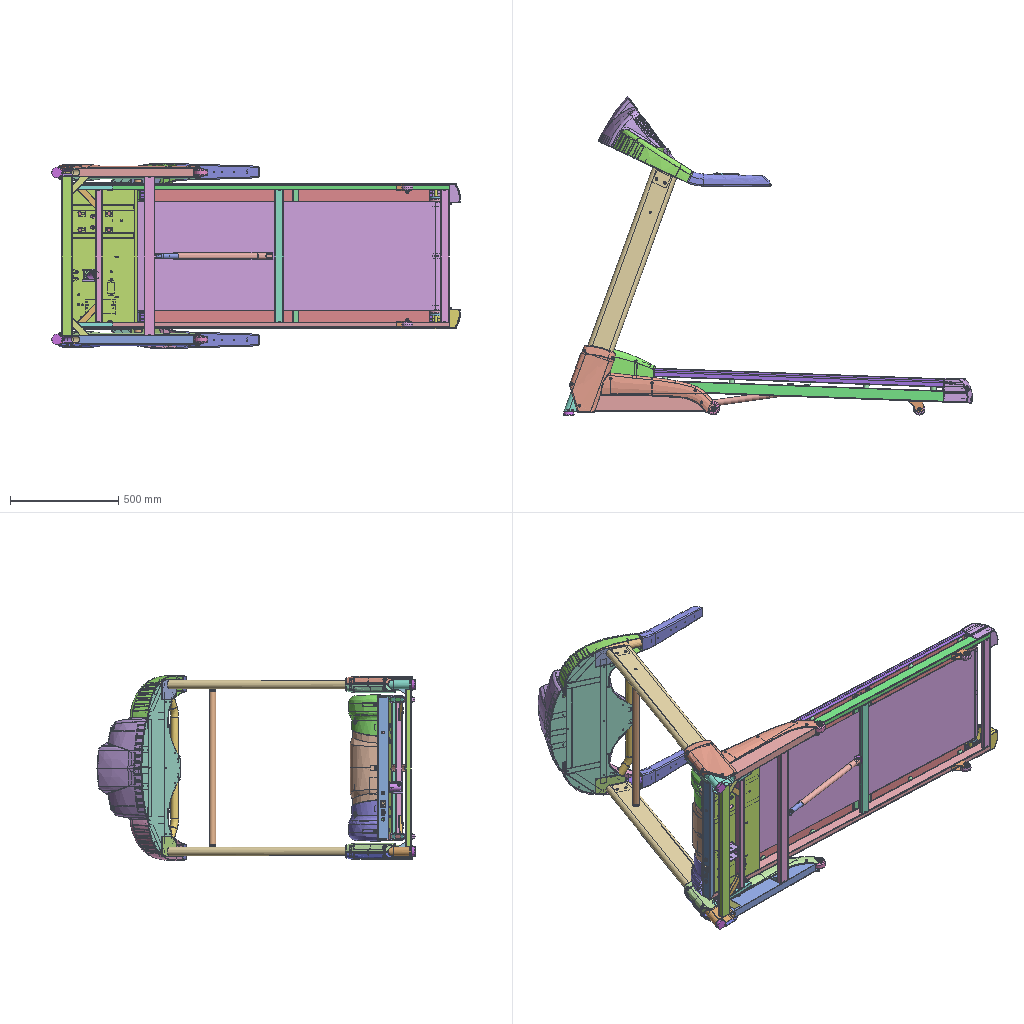Assembly | STEP file | 128 different items | 245 placed | box 1886 x 1467 x 856 mm
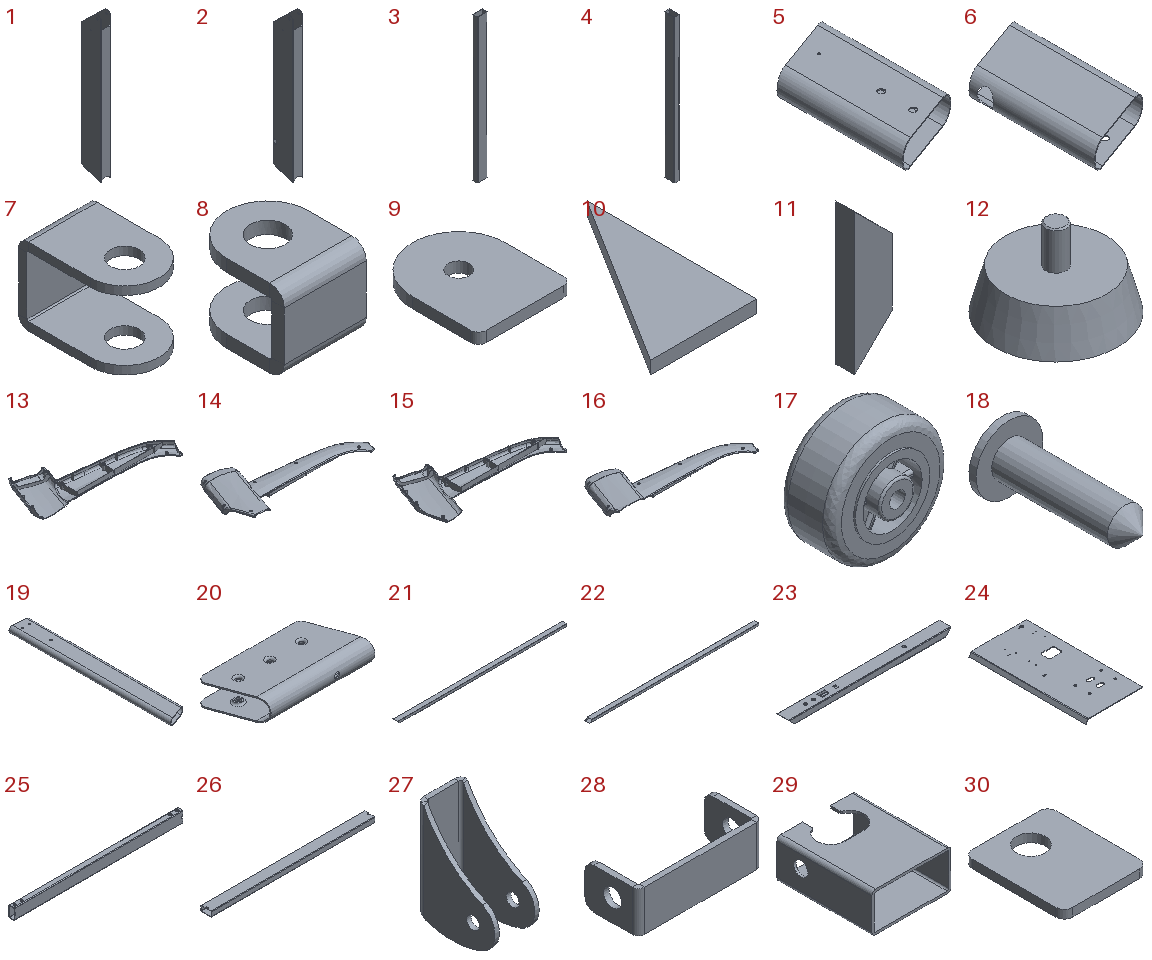Parts list (item | name | quantity | parent item | size | volume):
1 | Q7C0101L | x1 | in Q7C0100 | 40 x 80 x 584.662 mm | 247480 mm3
2 | Q7C0101R | x1 | in Q7C0100 | 40 x 80 x 584.662 mm | 247142 mm3
3 | PN_0025_default | x1 | in Q7C0100 | 50 x 25 x 730 mm | 154272 mm3
4 | PN_0006_default | x1 | in Q7C0100 | 25 x 50 x 730 mm | 154272 mm3
5 | Q7C0104L | x1 | in Q7C0100 | 120 x 240.676 x 40 mm | 82650 mm3
6 | Q7C0104R | x1 | in Q7C0100 | 120 x 240.549 x 40 mm | 81709 mm3
7 | Q7C0106 | x4 | in Q7C0100, Q7C0500 | 25 x 38.5 x 28 mm | 6374 mm3
8 | PN_0005_default | x1 | in Q7C0100 | 20 x 24 x 19 mm | 2959 mm3
9 | PN_0009_default | x2 | in Q7C0100 | 35 x 42.5 x 4 mm | 5208 mm3
10 | Q7C0109 | x4 | in Q7C0100 | 25 x 40 x 3 mm | 1500 mm3
11 | Q7C0110 | x2 | in Q7C0100 | 30 x 15 x 113 mm | 10458 mm3
12 | Q7C0102W | x2 | in Q7C0100Z | 48.593 x 48.593 x 32 mm | 27204 mm3
13 | PR12S0312~665.310.45LR | x1 | in Q7C0100Z | 660.94 x 308.881 x 43 mm | 303745 mm3
14 | PR12S0313~665.310.45LL | x1 | in Q7C0100Z | 660.94 x 308.908 x 43 mm | 328028 mm3
15 | PR12S0312~665.310.45RR | x1 | in Q7C0100Z | 660.94 x 308.908 x 43 mm | 328301 mm3
16 | PR12S0312~665.310.45RL | x1 | in Q7C0100Z | 660.94 x 308.881 x 43 mm | 302873 mm3
17 | 04FS0060~8.2.62.T35 | x2 | in Q7C0100Z | 62 x 35 x 62 mm | 74583 mm3
18 | ZG0415 | x1 | in Q7C0100Z | 7.5 x 16.961 x 7.5 mm | 227.201 mm3
19 | Q7C0201 | x2 | in Q7C0200 | 120 x 1000 x 40 mm | 489501 mm3
20 | PN_0014_default | x2 | in Q7C0200 | 192.331 x 89 x 35 mm | 64591 mm3
21 | Q7C0501L | x1 | in Q7C0500 | 1765 x 50 x 25 mm | 371060 mm3
22 | Q7C0501R | x1 | in Q7C0500 | 1765 x 50 x 25 mm | 371163 mm3
23 | Q7C0502 | x1 | in Q7C0500 | 658 x 50 x 25 mm | 125904 mm3
24 | PN_0024_default | x1 | in Q7C0500 | 299.634 x 609 x 21.187 mm | 548707 mm3
25 | Q7C0504 | x1 | in Q7C0500 | 610 x 20 x 40 mm | 101740 mm3
26 | Q7C0505 | x1 | in Q7C0500 | 610 x 40 x 20 mm | 101443 mm3
27 | Q7C0506 | x2 | in Q7C0500 | 30 x 53 x 70.522 mm | 17329 mm3
28 | Q7C0507 | x2 | in Q7C0500 | 70 x 30 x 23 mm | 7902 mm3
29 | Q7C0508 | x1 | in Q7C0500 | 50 x 60 x 25 mm | 11629 mm3
30 | Q7C0509 | x1 | in Q7C0500 | 50 x 60 x 5 mm | 13731 mm3
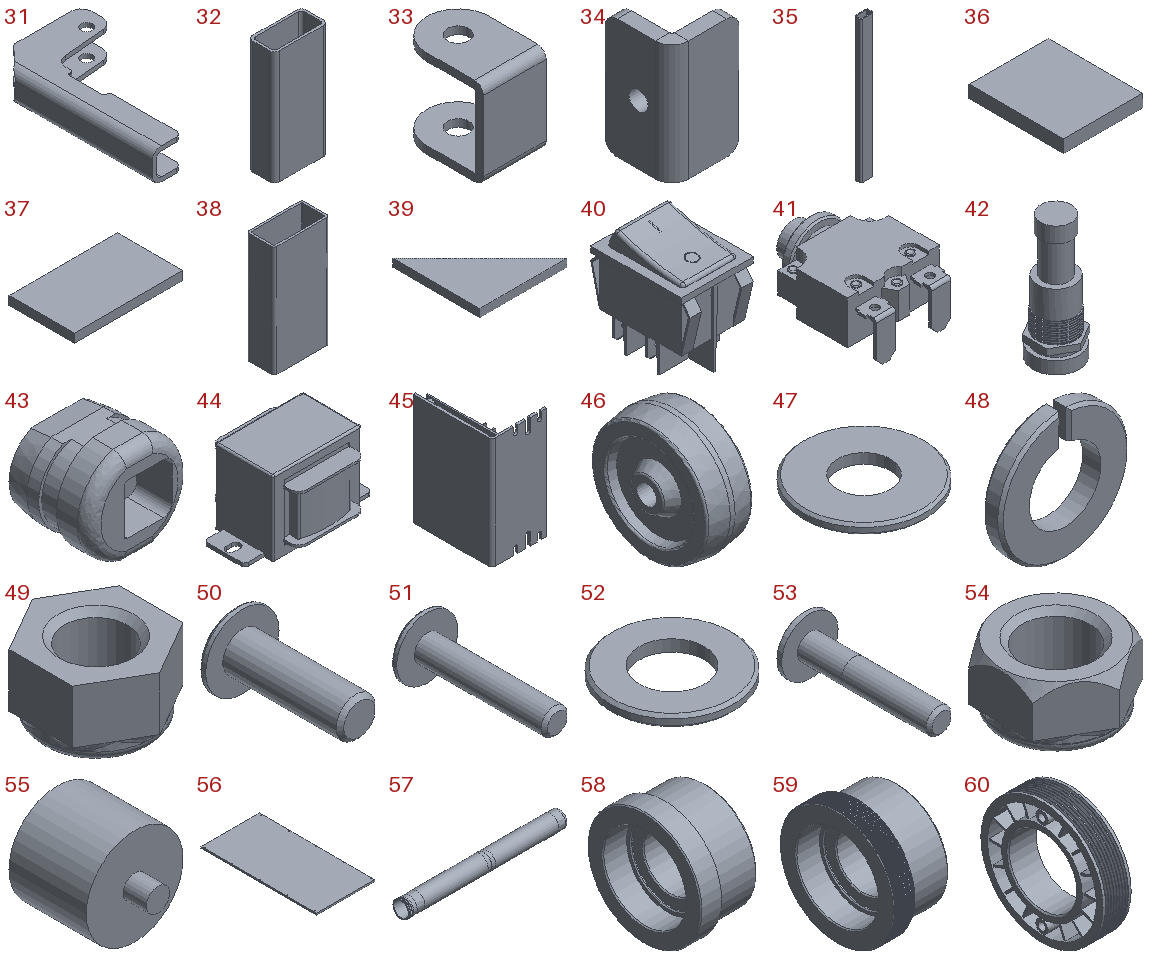31 | Q7C0510 | x1 | in Q7C0500 | 84 x 150 x 29 mm | 50454 mm3
32 | Q7C0511 | x2 | in Q7C0500 | 26 x 13 x 55 mm | 4616 mm3
33 | Q7C0512 | x1 | in Q7C0500 | 25 x 35 x 35 mm | 6553 mm3
34 | Q7C0513 | x7 | in Q7C0500 | 14 x 14 x 25 mm | 1757 mm3
35 | Q7C0515 | x2 | in Q7C0500 | 26 x 13 x 285 mm | 23919 mm3
36 | Q7C0516 | x1 | in Q7C0500 | 25 x 30 x 4 mm | 3000 mm3
37 | Q7C0518 | x2 | in Q7C0500 | 50 x 30 x 4 mm | 6000 mm3
38 | Q7C0519 | x1 | in Q7C0500 | 40 x 20 x 80 mm | 13422 mm3
39 | Q7C0517 | x2 | in Q7C0500 | 45 x 45 x 4 mm | 4050 mm3
40 | EP002 | x1 | in Q7C0500Z | 25 x 34.5 x 34.784 mm | 14567 mm3
41 | EC002 | x1 | in Q7C0500Z | 29.3 x 39.3 x 19.65 mm | 10331 mm3
42 | PN_0007_default | x1 | in Q7C0500Z | 15 x 16.018 x 40 mm | 4012 mm3
43 | PN_0016_default | x1 | in Q7C0500Z | 17 x 14 x 16 mm | 1519 mm3
44 | PN_0019-default | x1 | in Q7C0500Z | 72 x 50 x 42 mm | 79868 mm3
45 | ZY03WYF | x1 | in Q7C0500Z | 68 x 97.5 x 138 mm | 146420 mm3
46 | PN_0013_config | x2 | in Q7C0500Z | 22 x 52.843 x 52.843 mm | 34026 mm3
47 | PN_0027_config | x7 | in Q7C0500Z | 9.8 x 9.8 x 0.8 mm | 48.045 mm3
48 | W204009 | x7 | in Q7C0500Z | 9.2 x 1.3 x 9.193 mm | 57.255 mm3
49 | PN_0001_config | x8 | in Q7C0500Z | 7 x 8.083 x 4.7 mm | 129.872 mm3
50 | SD10412 | x9 | in Q7C0500Z | 9.4 x 17.503 x 9.4 mm | 388.67 mm3
51 | SD10420 | x2 | in Q7C0500Z | 9.4 x 22.503 x 9.4 mm | 345.867 mm3
52 | PN_0008_config | x5 | in Q7C0500Z | 17 x 17 x 1.6 mm | 252.969 mm3
53 | PN_0004_config | x3 | in Q7C0500Z, Q7C | 18 x 46.451 x 18 mm | 2805 mm3
54 | PN_0010_config | x2 | in Q7C0500Z | 13.017 x 15.011 x 7.5 mm | 666.866 mm3
55 | DECH01 | x8 | in Q7C0500Z | 25 x 26 x 25 mm | 9704 mm3
56 | DECAK NQ7A | x1 | in Q7C0500Z | 658 x 1310 x 18 mm | 15510409 mm3
57 | PN_0023_default | x1 | in Q7C0700ZA | 543 x 56 x 56 mm | 266273 mm3
58 | PN_0020_default | x1 | in Q7C0700ZA | 30 x 55.001 x 55.001 mm | 38129 mm3
59 | PN_0015_default | x1 | in Q7C0700ZA | 30 x 55.999 x 56 mm | 38879 mm3
60 | PN_0017_default | x1 | in Q7C0700ZA | 23 x 100 x 100 mm | 79245 mm3
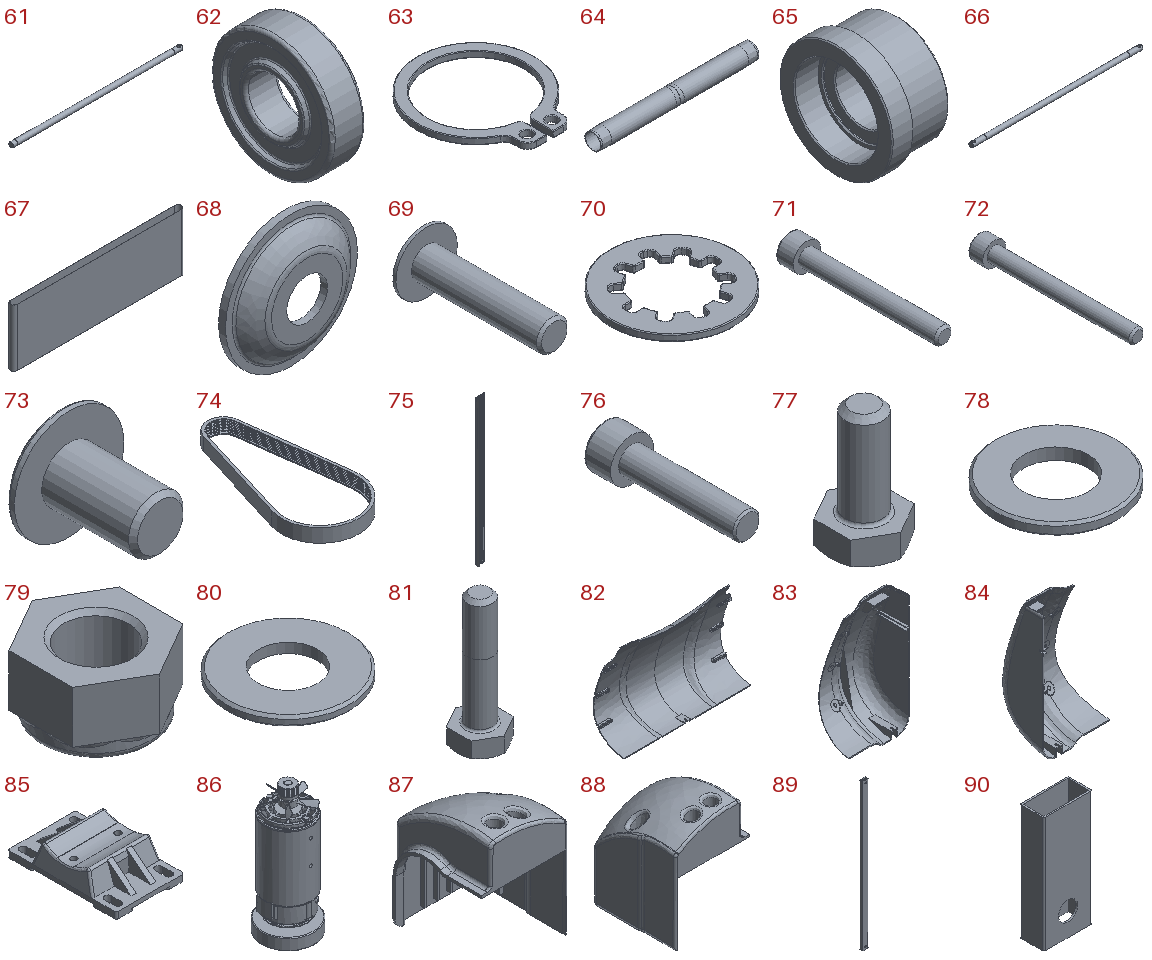61 | Q7C0702 | x1 | in Q7C0700Z | 610 x 17 x 17 mm | 138904 mm3
62 | PL6203ZZA_default | x4 | in Q7C0700Z, Q7C0800Z | 11 x 40 x 40 mm | 9892 mm3
63 | PN_0018_config | x4 | in Q7C0700Z, Q7C0800Z | 19 x 21.5 x 1 mm | 101.865 mm3
64 | PN_0012_default | x1 | in Q7C0800ZA | 530 x 56 x 56 mm | 259272 mm3
65 | PN_0003_default | x2 | in Q7C0800ZA | 30 x 54.43 x 54.43 mm | 37639 mm3
66 | Q7C0803 | x1 | in Q7C0800Z | 655 x 17 x 17 mm | 147236 mm3
67 | RUBE Q7C | x1 | in Q7C0500Z | 1492 x 59.6 x 500 mm | 2741026 mm3
68 | PN_0022_default | x6 | in Q7C0500Z | 21 x 3.607 x 21 mm | 386.807 mm3
69 | SD10625 | x8 | in Q7C0500Z | 12 x 27.352 x 12 mm | 852.352 mm3
70 | PN_0026_config | x3 | in Q7C0500Z | 15 x 15 x 0.8 mm | 82.689 mm3
71 | SA10865 | x1 | in Q7C0500Z | 13 x 73 x 13 mm | 4160 mm3
72 | SA10880 | x2 | in Q7C0500Z | 13 x 88 x 13 mm | 4914 mm3
73 | SD10610 | x5 | in Q7C0500Z | 12 x 12.964 x 12 mm | 479.053 mm3
74 | DE200JNQ7A | x1 | in Q7C0500Z | 103 x 213.3 x 18 mm | 21815 mm3
75 | SIDE-D default | x2 | in Q7C0500Z | 82 x 38 x 1350 mm | 698294 mm3
76 | SA10835 | x1 | in Q7C0500Z | 13 x 43 x 13 mm | 2660 mm3
77 | SI1025_M10 | x4 | in Q7C0500Z | 17 x 19.6 x 32 mm | 3678 mm3
78 | PN_0028_config | x5 | in Q7C0500Z | 21 x 21 x 2 mm | 492.233 mm3
79 | N210095 | x5 | in Q7C0500Z | 17 x 19.63 x 10.5 mm | 1722 mm3
80 | PN_0021_config | x1 | in Q7C0500Z | 25 x 25 x 2 mm | 736.18 mm3
81 | SI11045_M10 | x1 | in Q7C0500Z | 17 x 19.6 x 52 mm | 5249 mm3
82 | MOTOR COVER Z | x1 | in Q7C0500Z | 500 x 131.956 x 336.482 mm | 623732 mm3
83 | MOTOR COVER R | x1 | in Q7C0500Z | 191.608 x 140.54 x 371.606 mm | 329037 mm3
84 | MOTOR COVER L | x1 | in Q7C0500Z | 191.608 x 140.54 x 371.606 mm | 339460 mm3
85 | MDZ Q7A | x1 | in Q7C0600Z | 100 x 160 x 38.7 mm | 142621 mm3
86 | MOTOR Q7A | x1 | in Q7C0600Z | 142 x 142 x 347 mm | 1832785 mm3
87 | EDN CAP NQ7A | x1 | in Q7C0500Z | 100.427 x 109.896 x 135.338 mm | 139649 mm3
88 | EDN CAP NQ7AL | x1 | in Q7C0500Z | 100.427 x 109.896 x 135.338 mm | 140123 mm3
89 | Q7C0901 | x2 | in Q7C0500Z | 26 x 13 x 648 mm | 67252 mm3
90 | Q7C1201 | x2 | in Q7C1200 | 30 x 15 x 72 mm | 5997 mm3
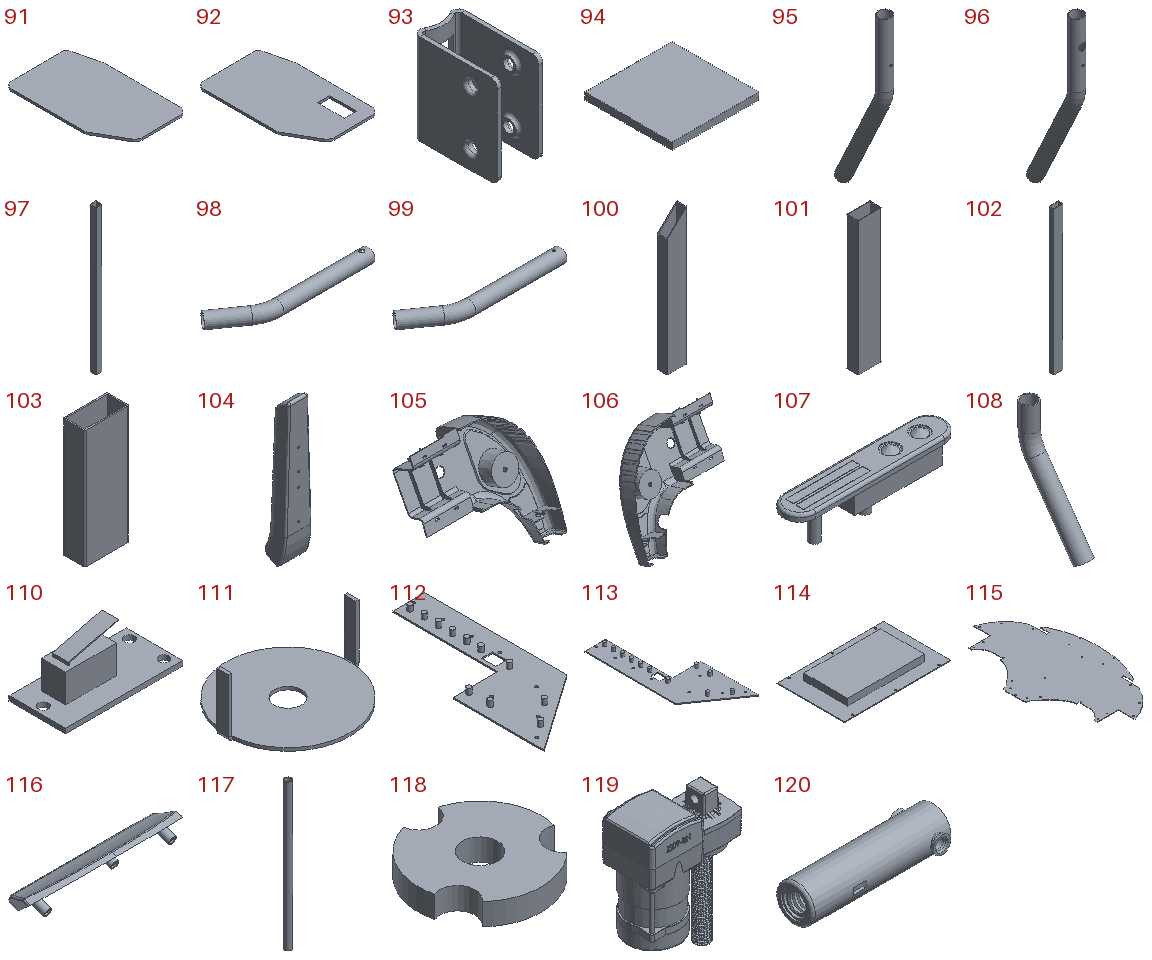91 | Q7C1202L | x1 | in Q7C1200 | 90 x 149 x 3 mm | 37856 mm3
92 | Q7C1202R | x1 | in Q7C1200 | 90 x 149 x 3 mm | 36176 mm3
93 | PN_0011_default | x2 | in Q7C1200 | 35 x 65 x 70 mm | 31433 mm3
94 | Q7C1204 | x2 | in Q7C1200 | 25 x 25 x 2 mm | 1250 mm3
95 | Q7C1205L | x1 | in Q7C1200 | 38.1 x 161.362 x 488.383 mm | 85140 mm3
96 | Q7C1205R | x1 | in Q7C1200 | 38.1 x 161.362 x 488.383 mm | 84651 mm3
97 | Q7C1206 | x1 | in Q7C1200 | 30 x 30 x 700 mm | 154296 mm3
98 | Q7C1207L | x1 | in Q7C1200 | 330.538 x 89.278 x 31.8 mm | 48236 mm3
99 | Q7C1207R | x1 | in Q7C1200 | 330.538 x 89.278 x 31.8 mm | 48237 mm3
100 | Q7C1208 | x2 | in Q7C1200 | 30 x 15 x 209.35 mm | 16574 mm3
101 | Q7C1209 | x2 | in Q7C1200 | 30 x 15 x 169 mm | 14389 mm3
102 | Q7C1210 | x1 | in Q7C1200 | 30 x 15 x 450 mm | 38263 mm3
103 | Q7C1211 | x1 | in Q7C1200 | 30 x 15 x 80 mm | 6811 mm3
104 | Handlebar Cover L | x2 | in Q7C1200ZB | 78.327 x 65.639 x 387.41 mm | 737396 mm3
105 | Consen Cover L | x1 | in Q7C1200ZB | 398.708 x 218.09 x 381.338 mm | 579816 mm3
106 | Consen Cover R | x1 | in Q7C1200ZB | 398.708 x 218.09 x 381.338 mm | 568981 mm3
107 | Q7C1216W | x2 | in Q7C1200ZB | 119.5 x 24 x 32.509 mm | 28513 mm3
108 | Q7C1217W | x2 | in Q7C1200ZB | 35.8 x 156.01 x 266.792 mm | 62409 mm3
109 | Consen Cover | x1 | in Q7C1200ZA | - | -
110 | Q7C1213W | x1 | in Q7C1200ZA | 29 x 14 x 12 mm | 1005 mm3
111 | Q7C1215W | x1 | in Q7C1200ZA | 33.859 x 32 x 15.058 mm | 684.385 mm3
112 | PCB-R | x1 | in Q7C1200ZA | 108 x 276 x 10 mm | 34872 mm3
113 | PCB-L | x1 | in Q7C1200ZA | 108 x 276 x 10 mm | 34872 mm3
114 | Q7C1214W | x1 | in Q7C1200ZA | 223 x 140 x 15.5 mm | 251677 mm3
115 | Rear Consen Cover | x1 | in Q7C1200Z | 420.328 x 794.391 x 2 mm | 399134 mm3
116 | 50FAS0309~100.33.15 | x1 | in Q7C1200Z | - | -
117 | Q7C1301 | x1 | in Q7C1300 | 31.8 x 31.8 x 726 mm | 103662 mm3
118 | PN_0002_default | x2 | in Q7C1300 | 28 x 27.429 x 5 mm | 2473 mm3
119 | JS-09 Q7A | x1 | in Q7C | 127.975 x 72.828 x 177.5 mm | 665707 mm3
120 | JS09-BNB Q7A | x1 | in Q7C | 130.5 x 41.999 x 35 mm | 51748 mm3
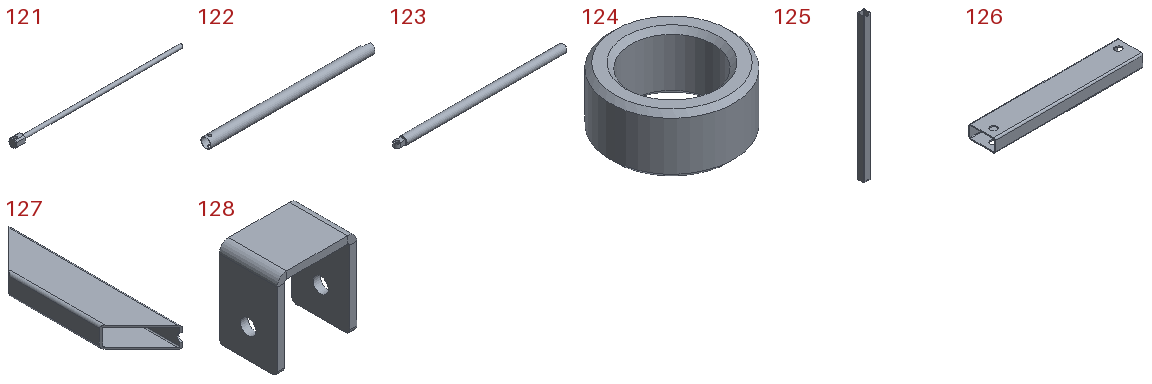121 | GAS SHOCK Q7AS | x1 | in Q7C | 478.5 x 20 x 20 mm | 44511 mm3
122 | GAS SHOCK Q7AW | x1 | in Q7C | 460 x 28 x 28 mm | 56023 mm3
123 | GAS SHOCK Q7AX | x1 | in Q7C | 474 x 22 x 22 mm | 124828 mm3
124 | Q7C0902 | x1 | in Q7C | 12.7 x 12.7 x 6 mm | 402.941 mm3
125 | PN_0030_default | x1 | in Q7C0400 | 30 x 30 x 612 mm | 101776 mm3
126 | Q7C0402 | x2 | in Q7C0400 | 225 x 40 x 20 mm | 36971 mm3
127 | Q7C0403 | x2 | in Q7C0400 | 30 x 125 x 15 mm | 9413 mm3
128 | Q7C0404 | x1 | in Q7C0400 | 55 x 40 x 60 mm | 31409 mm3
Placements (level | parent | child | x y z in mm | rotation matrix by rows):
1 | Q7C | Q7C0100Z | -0.0 -0.0 -0.0 | 1 0 0 0 1 0 0 0 1
2 | Q7C0100Z | Q7C0100 | -0.0 -0.0 -0.0 | 1 0 0 0 1 0 0 0 1
3 | Q7C0100 | Q7C0101L | -535.0 27.5 350.0 | 0 0 1 0 1 0 -1 0 -0
3 | Q7C0100 | Q7C0101R | -535.0 27.5 -460.0 | 0 0 1 0 1 0 -1 0 -0
3 | Q7C0100 | PN_0025_default | -581.109 40.0 -55.0 | -1 0 0 0 -1 0 0 0 1
3 | Q7C0100 | PN_0006_default | -188.608 52.5 -55.0 | 0 -1 0 1 0 0 0 0 1
3 | Q7C0100 | Q7C0104L | -560.746 99.538 330.0 | -0.9397 -0.342 0 0.342 -0.9397 0 0 0 1
3 | Q7C0100 | Q7C0104R | -560.724 99.598 -440.0 | -0.9397 -0.342 0 0.342 -0.9397 0 0 0 1
3 | Q7C0100 | Q7C0106 | -595.109 52.5 247.0 | 1 0 0 0 -1 0 0 0 -1
3 | Q7C0100 | Q7C0106 | -570.109 52.5 -357.0 | -1 0 0 0 -1 0 0 0 1
3 | Q7C0100 | PN_0005_default | -176.108 37.5 -55.0 | 0 1 0 -1 0 0 0 0 1
3 | Q7C0100 | PN_0009_default | -628.489 30.5 329.8 | 0 -1 0 0 0 1 -1 0 0
3 | Q7C0100 | PN_0009_default | -628.489 30.5 -440.2 | 0 -1 0 0 0 1 -1 0 0
3 | Q7C0100 | Q7C0109 | -226.108 52.5 -420.0 | 0 0 1 0 1 0 -1 0 -0
3 | Q7C0100 | Q7C0109 | -179.108 52.5 -420.0 | 0 0 1 0 1 0 -1 0 -0
3 | Q7C0100 | Q7C0109 | -176.108 52.5 310.0 | 0 0 -1 0 1 0 1 0 0
3 | Q7C0100 | Q7C0109 | -223.108 52.5 310.0 | 0 0 -1 0 1 0 1 0 0
3 | Q7C0100 | Q7C0110 | -566.715 45.0 -350.704 | -0.7071 0 0.7071 0 1 0 -0.7071 0 -0.7071
3 | Q7C0100 | Q7C0110 | -486.812 45.0 320.607 | -0.7071 0 -0.7071 0 1 0 0.7071 0 -0.7071
2 | Q7C0100Z | Q7C0102W | -628.489 27.5 329.8 | 0.9959 0.09062 0 0 0 1 0.09062 -0.9959 0
2 | Q7C0100Z | Q7C0102W | -628.489 27.619 -440.2 | 0.3004 0.9538 0 0 0 1 0.9538 -0.3004 0
2 | Q7C0100Z | PR12S0312~665.310.45LR | -614.995 22.5 330.5 | 1 0 0 0 1 0 0 0 1
2 | Q7C0100Z | PR12S0313~665.310.45LL | -614.995 22.5 329.5 | 1 0 0 0 1 0 0 0 1
2 | Q7C0100Z | PR12S0312~665.310.45RR | -614.951 22.619 -439.5 | 1 0 0 0 1 0 0 0 1
2 | Q7C0100Z | PR12S0312~665.310.45RL | -614.951 22.619 -440.5 | 1 0 0 0 1 0 0 0 1
2 | Q7C0100Z | 04FS0060~8.2.62.T35 | 37.0 42.5 330.0 | 0.7571 0 -0.6533 0.6533 0 0.7571 0 -1 0
2 | Q7C0100Z | 04FS0060~8.2.62.T35 | 37.0 42.5 -440.0 | -0.9894 0 0.1451 -0.1451 0 -0.9894 0 -1 -0
2 | Q7C0100Z | ZG0415 | -445.0 92.5 320.0 | 0.9281 0 -0.3722 0 1 0 0.3722 0 0.9281
1 | Q7C | Q7C0200 | -358.863 603.056 350.0 | 0.9397 0.342 0 -0.342 0.9397 0 0 0 1
2 | Q7C0200 | Q7C0201 | -17.495 -442.636 -20.0 | 1 0 0 0 1 0 0 0 1
2 | Q7C0200 | PN_0014_default | 14.005 -355.575 -37.5 | 0 1 0 -1 0 0 0 0 1
1 | Q7C | Q7C0200 | -358.863 603.056 -420.0 | 0.9397 0.342 0 -0.342 0.9397 0 0 0 1
2 | Q7C0200 | Q7C0201 | -17.495 -442.636 -20.0 | 1 0 0 0 1 0 0 0 1
2 | Q7C0200 | PN_0014_default | 14.005 -355.575 -37.5 | 0 1 0 -1 0 0 0 0 1
1 | Q7C | Q7C0500Z | 190.657 193.703 277.959 | 0.9993 0.03666 0 -0.03666 0.9993 0 0 0 1
2 | Q7C0500Z | Q7C0500 | -0.0 -0.0 -0.0 | 1 0 0 0 1 0 0 0 1
3 | Q7C0500 | Q7C0501L | 112.255 -64.436 -15.459 | 1 0 0 0 1 0 0 0 1
3 | Q7C0500 | Q7C0501R | 112.255 -64.436 -650.459 | 1 0 0 0 1 0 0 0 1
3 | Q7C0500 | Q7C0502 | -757.745 -64.436 -332.959 | 0 0 -1 0 1 0 1 0 0
3 | Q7C0500 | PN_0024_default | -745.245 -86.436 -332.959 | -1 0 0 0 0 -1 0 -1 0
3 | Q7C0500 | Q7C0504 | 974.755 -79.436 -332.959 | 0 0 1 0 1 0 -1 0 -0
3 | Q7C0500 | Q7C0505 | 209.755 -79.436 -332.959 | 0 -1 0 0 0 -1 1 0 0
3 | Q7C0500 | Q7C0506 | 791.255 -89.436 -17.959 | 0 0 -1 0 1 0 1 0 -0
3 | Q7C0500 | Q7C0506 | 791.255 -89.436 -647.959 | 0 0 -1 0 1 0 1 0 -0
3 | Q7C0500 | Q7C0507 | 949.755 -24.436 -16.459 | 1 0 0 0 1 0 0 0 1
3 | Q7C0500 | Q7C0507 | 949.755 -24.436 -649.459 | -1 0 0 0 1 0 0 0 -1
3 | Q7C0500 | Q7C0508 | -500.245 -39.436 -625.459 | 1 0 0 0 1 0 0 0 1
3 | Q7C0500 | Q7C0509 | -500.245 -69.436 -32.959 | 1 0 0 0 1 0 0 0 1
3 | Q7C0500 | Q7C0510 | -724.245 63.564 -421.959 | 1 0 0 0 1 0 0 0 1
3 | Q7C0500 | Q7C0511 | -440.745 -11.936 -649.959 | 0 1 0 0 0 -1 -1 0 0
3 | Q7C0500 | Q7C0511 | -440.745 -11.936 -15.959 | 0 1 0 0 0 -1 -1 0 0
3 | Q7C0500 | Q7C0512 | 189.755 -76.936 -332.959 | 0 -1 0 1 0 0 0 0 1
3 | Q7C0500 | Q7C0513 | -510.245 -39.436 -659.959 | 0 0 -1 0 1 0 1 0 0
3 | Q7C0500 | Q7C0513 | -767.245 -39.436 -623.959 | 1 0 0 0 1 0 0 0 1
3 | Q7C0500 | Q7C0513 | -767.245 -39.436 -332.959 | 1 0 0 0 1 0 0 0 1
3 | Q7C0500 | Q7C0513 | -767.245 -39.436 -41.959 | 1 0 0 0 1 0 0 0 1
3 | Q7C0500 | Q7C0513 | -510.245 -39.436 -5.959 | 0 0 1 0 1 0 -1 0 -0
3 | Q7C0500 | Q7C0515 | -602.745 -79.936 -110.459 | 0 0 1 0 1 0 -1 0 0
3 | Q7C0500 | Q7C0515 | -602.745 -79.936 -238.459 | 0 0 1 0 1 0 -1 0 0
3 | Q7C0500 | Q7C0516 | -725.245 67.564 -407.459 | -1 0 0 0 0 -1 0 -1 0
3 | Q7C0500 | Q7C0106 | -582.745 -89.436 -634.959 | 1 0 0 0 1 0 0 0 1
3 | Q7C0500 | Q7C0106 | -557.745 -89.436 -30.959 | -1 0 0 0 1 0 0 0 -1
3 | Q7C0500 | Q7C0513 | -767.245 -39.436 -145.459 | 0 1 0 1 0 0 0 0 -1
3 | Q7C0500 | Q7C0513 | -767.245 -39.436 -520.459 | 0 1 0 1 0 0 0 0 -1
3 | Q7C0500 | Q7C0518 | -732.341 -61.436 -402.328 | 0 0.9397 0.342 -1 0 0 0 -0.342 0.9397
3 | Q7C0500 | Q7C0518 | -730.149 -61.436 -446.423 | 0 0.9063 -0.4226 -1 0 0 0 0.4226 0.9063
3 | Q7C0500 | Q7C0519 | -755.245 -19.436 -457.459 | 0 1 0 -1 0 0 0 0 1
3 | Q7C0500 | Q7C0517 | -745.245 -43.436 -637.959 | 0 1 0 0 0 1 1 0 -0
3 | Q7C0500 | Q7C0517 | -745.245 -43.436 -27.959 | 1 0 0 0 0 1 0 -1 0
2 | Q7C0500Z | EP002 | -770.245 -64.686 -497.909 | 0 0 -1 -1 0 0 0 1 0
2 | Q7C0500Z | EC002 | -712.965 -71.336 -495.294 | 0 -1 0 0 0 -1 1 0 0
2 | Q7C0500Z | PN_0007_default | -734.245 -64.436 -569.959 | 0 0 1 0 1 0 -1 0 -0
2 | Q7C0500Z | PN_0016_default | -775.745 -63.161 -447.959 | 0 1 0 1 0 0 0 0 -1
2 | Q7C0500Z | PN_0019-default | -581.745 -86.436 -454.959 | 0 -1 0 0 0 1 -1 0 0
2 | Q7C0500Z | ZY03WYF | -616.245 -86.436 -602.959 | 0 0 -1 0 1 0 1 0 -0
2 | Q7C0500Z | PN_0013_config | 802.755 -127.436 -17.959 | 0 -0.383 0.9237 0 0.9237 0.383 -1 0 0
2 | Q7C0500Z | PN_0013_config | 802.755 -127.436 -647.959 | 0 0.9578 -0.2876 0 -0.2876 -0.9578 -1 0 0
2 | Q7C0500Z | PN_0027_config | -565.245 -83.636 -512.459 | 1 0 0 0 0 -1 0 1 -0
2 | Q7C0500Z | PN_0027_config | -715.245 -86.436 -512.459 | 1 0 0 0 0 1 0 -1 0
2 | Q7C0500Z | PN_0027_config | -565.245 -86.436 -405.459 | 1 0 0 0 0 1 0 -1 0
2 | Q7C0500Z | PN_0027_config | -555.245 -83.436 -557.459 | 1 0 0 0 0 1 0 -1 0
2 | Q7C0500Z | PN_0027_config | -698.245 -83.436 -557.459 | 1 0 0 0 0 1 0 -1 0
2 | Q7C0500Z | W204009 | -565.245 -83.636 -512.459 | -0.2314 0 0.9729 0 1 0 -0.9729 0 -0.2314
2 | Q7C0500Z | W204009 | -715.245 -84.336 -512.459 | 1 0 0 0 -1 0 0 0 -1
2 | Q7C0500Z | W204009 | -565.245 -85.636 -405.459 | -0.1182 0 -0.993 0 1 0 0.993 0 -0.1182
2 | Q7C0500Z | W204009 | -555.245 -81.336 -557.459 | 1 0 0 0 -1 0 0 0 -1
2 | Q7C0500Z | W204009 | -698.245 -81.336 -557.459 | 1 0 0 0 -1 0 0 0 -1
2 | Q7C0500Z | PN_0001_config | -698.245 -92.836 -557.459 | 1 0 0 0 0 1 0 -1 -0
2 | Q7C0500Z | PN_0001_config | -610.245 -92.836 -512.459 | 1 0 0 0 0 1 0 -1 -0
2 | Q7C0500Z | PN_0001_config | -715.245 -92.836 -512.459 | 1 0 0 0 0 1 0 -1 -0
2 | Q7C0500Z | PN_0001_config | -565.245 -92.836 -512.459 | 1 0 0 0 0 1 0 -1 -0
2 | Q7C0500Z | PN_0001_config | -555.245 -92.836 -557.459 | 1 0 0 0 0 1 0 -1 -0
2 | Q7C0500Z | PN_0001_config | -565.245 -92.836 -405.459 | -0.985 0.1727 0 0 0 1 0.1727 0.985 -0
2 | Q7C0500Z | SD10412 | -565.245 -84.336 -405.459 | -0.9996 0 0.02688 0 1 0 -0.02688 0 -0.9996
2 | Q7C0500Z | SD10412 | -715.245 -84.336 -512.459 | 0.6319 0 0.775 0 1 0 -0.775 0 0.6319
2 | Q7C0500Z | SD10412 | -565.245 -82.336 -512.459 | -0.7618 0 -0.6478 0 1 0 0.6478 0 -0.7618
2 | Q7C0500Z | SD10420 | -698.245 -81.336 -557.459 | 0.9278 0 0.3732 0 1 0 -0.3732 0 0.9278
2 | Q7C0500Z | SD10420 | -555.245 -81.336 -557.459 | 0.8397 0 0.543 0 1 0 -0.543 0 0.8397
2 | Q7C0500Z | SD10412 | -565.245 -82.336 -441.459 | 1 0 0 0 1 0 0 0 1
2 | Q7C0500Z | PN_0001_config | -565.245 -92.836 -441.459 | 1 0 0 0 0 1 0 -1 -0
2 | Q7C0500Z | PN_0027_config | -565.245 -84.436 -441.459 | 1 0 0 0 0 1 0 -1 0
2 | Q7C0500Z | W204009 | -565.245 -82.336 -441.459 | 1 0 0 0 -1 0 0 0 -1
2 | Q7C0500Z | PN_0008_config | 802.755 -127.436 -34.559 | 0.9837 0.1797 0 -0.1797 0.9837 0 0 0 1
2 | Q7C0500Z | PN_0008_config | 802.755 -127.436 -631.359 | 0.9528 -0.3036 0 -0.3036 -0.9528 0 0 0 -1
2 | Q7C0500Z | PN_0004_config | 802.755 -127.436 -2.959 | 1 0 0 0 0 -1 0 1 -0
2 | Q7C0500Z | PN_0004_config | 802.755 -127.436 -662.959 | 0.9981 0 0.06117 -0.06117 0 0.9981 0 -1 -0
2 | Q7C0500Z | PN_0010_config | 802.755 -127.436 -40.059 | 1 0 0 0 1 0 0 0 1
2 | Q7C0500Z | PN_0010_config | 802.755 -127.436 -625.859 | -0.9237 -0.383 0 -0.383 0.9237 0 0 0 -1
2 | Q7C0500Z | DECH01 | 864.755 -45.436 -15.459 | 0.8865 0 -0.4627 0 1 0 0.4627 0 0.8865
2 | Q7C0500Z | DECH01 | 864.755 -45.436 -650.459 | 0.8865 0 -0.4627 0 1 0 0.4627 0 0.8865
2 | Q7C0500Z | DECH01 | 554.755 -45.436 -15.459 | 0.8865 0 -0.4627 0 1 0 0.4627 0 0.8865
2 | Q7C0500Z | DECH01 | 554.755 -45.436 -650.459 | 0.8865 0 -0.4627 0 1 0 0.4627 0 0.8865
2 | Q7C0500Z | DECH01 | -65.245 -45.436 -15.459 | 0.8865 0 -0.4627 0 1 0 0.4627 0 0.8865
2 | Q7C0500Z | DECH01 | -65.245 -45.436 -650.459 | 0.8865 0 -0.4627 0 1 0 0.4627 0 0.8865
2 | Q7C0500Z | DECAK NQ7A | 244.755 -10.436 -332.959 | 0 -1 0 0 0 1 -1 0 -0
2 | Q7C0500Z | Q7C0700Z | -500.245 -24.436 -320.259 | 0 1 0 0 0 -1 -1 0 -0
3 | Q7C0700Z | Q7C0700ZA | 0.0 0.0 -0.0 | 1 0 0 0 1 0 0 0 1
4 | Q7C0700ZA | PN_0023_default | -0.0 -0.0 0.0 | 1 0 0 0 1 0 0 0 1
4 | Q7C0700ZA | PN_0020_default | 281.5 0.0 0.0 | -1 0 0 0 0.5057 -0.8627 0 -0.8627 -0.5057
4 | Q7C0700ZA | PN_0015_default | -281.5 0.0 0.0 | 1 0 0 0 1 0 0 0 1
4 | Q7C0700ZA | PN_0017_default | -281.5 0.0 0.0 | 1 0 0 0 1 0 0 0 1
3 | Q7C0700Z | Q7C0702 | -22.3 0.0 -0.0 | 1 0 0 0 0 1 0 -1 -0
3 | Q7C0700Z | PL6203ZZA_default | 270.5 8.5 -0.0 | 1 0 0 0 1 0 0 0 1
3 | Q7C0700Z | PL6203ZZA_default | -281.5 8.5 -0.0 | 1 0 0 0 1 0 0 0 1
3 | Q7C0700Z | PN_0018_config | 281.6 0.0 -0.0 | 0 0 1 0 1 0 -1 0 -0
3 | Q7C0700Z | PN_0018_config | -282.6 0.0 -0.0 | 0 0 1 0 1 0 -1 0 -0
2 | Q7C0500Z | Q7C0800Z | 931.755 -24.936 -332.959 | 0 0 -1 0 1 0 1 0 -0
3 | Q7C0800Z | Q7C0800ZA | -0.0 0.0 0.0 | 1 0 0 0 1 0 0 0 1
4 | Q7C0800ZA | PN_0012_default | 0.0 -0.0 -0.0 | 1 0 0 0 1 0 0 0 1
4 | Q7C0800ZA | PN_0003_default | -275.0 -0.0 0.0 | 1 0 0 0 1 0 0 0 1
4 | Q7C0800ZA | PN_0003_default | 275.0 -0.0 0.0 | -1 0 0 0 0.3818 -0.9242 0 -0.9242 -0.3818
3 | Q7C0800Z | PL6203ZZA_default | -275.0 8.5 -0.0 | 1 0 0 0 1 0 0 0 1
3 | Q7C0800Z | PL6203ZZA_default | 264.0 8.5 -0.0 | 1 0 0 0 1 0 0 0 1
3 | Q7C0800Z | PN_0018_config | 275.1 0.0 0.0 | 0 0 1 0 1 0 -1 0 0
3 | Q7C0800Z | PN_0018_config | -275.3 0.0 0.0 | 0 0 -1 0 1 0 1 0 0
3 | Q7C0800Z | Q7C0803 | -0.0 0.0 0.0 | 1 0 0 0 1 0 0 0 1
2 | Q7C0500Z | RUBE Q7C | 748.255 -24.872 -332.959 | 1 0.000349 0 -0.000349 1 0 0 0 1
2 | Q7C0500Z | PN_0022_default | 864.755 -1.389 -15.459 | 0.1704 0 -0.9854 0 1 0 0.9854 0 0.1704
2 | Q7C0500Z | PN_0022_default | 244.755 -1.389 -15.459 | 1 0 0.002792 0 1 0 -0.002792 0 1
2 | Q7C0500Z | PN_0022_default | -375.245 -1.389 -15.459 | 1 0 0 0 1 0 0 0 1
2 | Q7C0500Z | SD10625 | 864.755 0.4912 -15.459 | -0.5022 0 -0.8648 0 1 0 0.8648 0 -0.5022
2 | Q7C0500Z | SD10625 | 864.755 0.4912 -650.459 | -0.5022 0 -0.8648 0 1 0 0.8648 0 -0.5022
2 | Q7C0500Z | SD10625 | 554.755 0.4912 -15.459 | -0.5022 0 -0.8648 0 1 0 0.8648 0 -0.5022
2 | Q7C0500Z | SD10625 | 554.755 0.4912 -650.459 | -0.5022 0 -0.8648 0 1 0 0.8648 0 -0.5022
2 | Q7C0500Z | SD10625 | -65.245 0.4912 -15.459 | -0.5022 0 -0.8648 0 1 0 0.8648 0 -0.5022
2 | Q7C0500Z | SD10625 | -65.245 0.4912 -650.459 | -0.5022 0 -0.8648 0 1 0 0.8648 0 -0.5022
2 | Q7C0500Z | PN_0026_config | 985.555 -24.936 -15.459 | 0 0 -1 0 1 0 1 0 -0
2 | Q7C0500Z | PN_0026_config | -526.045 -24.436 -622.959 | 0 0 1 0 1 0 -1 0 0
2 | Q7C0500Z | PN_0008_config | 987.155 -24.936 -15.459 | 0 0 -1 0.9849 0.173 0 0.173 -0.9849 -0
2 | Q7C0500Z | PN_0008_config | -527.645 -24.436 -622.959 | 0 0 1 0 1 0 -1 0 0
2 | Q7C0500Z | SA10865 | -527.645 -24.436 -622.959 | 0 -1 0 1 0 0 0 0 1
2 | Q7C0500Z | SA10880 | 987.155 -24.936 -15.459 | 0 1 0 0.7886 0 0.6149 0.6149 0 -0.7886
2 | Q7C0500Z | PN_0022_default | -375.245 -1.389 -650.459 | 1 0 0 0 1 0 0 0 1
2 | Q7C0500Z | PN_0022_default | 244.755 -1.389 -650.459 | 1 0 0.002792 0 1 0 -0.002792 0 1
2 | Q7C0500Z | PN_0022_default | 864.755 -1.389 -650.459 | 0.1704 0 -0.9854 0 1 0 0.9854 0 0.1704
2 | Q7C0500Z | SD10412 | 999.755 -70.936 -38.959 | 0 1 0 -1 0 0 0 0 1
2 | Q7C0500Z | SD10412 | 999.755 -70.936 -601.959 | 0 1 0 0.3353 0 0.9421 0.9421 0 -0.3353
2 | Q7C0500Z | SD10610 | -510.245 -32.436 5.043 | -0.616 0 0.7878 0.7878 0 0.616 0 1 -0
2 | Q7C0500Z | SD10610 | -770.245 -32.436 -41.959 | 0 -1 0 0.9994 0 -0.03489 0.03489 0 0.9994
2 | Q7C0500Z | SD10610 | -773.245 -32.436 -332.959 | 0 -1 0 1 0 0 0 0 1
2 | Q7C0500Z | SD10610 | -770.245 -32.436 -623.959 | 0 -1 0 0.9994 0 0.03489 -0.03489 0 0.9994
2 | Q7C0500Z | SD10610 | -510.245 -32.436 -662.959 | -0.9199 0 0.3922 -0.3922 0 -0.9199 0 -1 -0
2 | Q7C0500Z | DE200JNQ7A | -168.442 429.736 -50.259 | 0.1283 -0.9917 0 0.9917 0.1283 0 0 0 1
2 | Q7C0500Z | DECH01 | -375.245 -45.436 -15.459 | 0.8865 0 -0.4627 0 1 0 0.4627 0 0.8865
2 | Q7C0500Z | DECH01 | -375.245 -45.436 -650.459 | 0.8865 0 -0.4627 0 1 0 0.4627 0 0.8865
2 | Q7C0500Z | SD10625 | -375.245 0.4912 -15.459 | -0.5022 0 -0.8648 0 1 0 0.8648 0 -0.5022
2 | Q7C0500Z | SD10625 | -375.245 0.4912 -650.459 | -0.5022 0 -0.8648 0 1 0 0.8648 0 -0.5022
2 | Q7C0500Z | SIDE-D default | 915.82 16.564 0.0413 | 0 0 1 0 1 0 -1 0 0
2 | Q7C0500Z | SIDE-D default | -434.18 16.564 -665.959 | 0 0 -1 0 1 0 1 0 0
2 | Q7C0500Z | PN_0026_config | 985.555 -24.936 -650.459 | 0 0 -1 0 1 0 1 0 -0
2 | Q7C0500Z | PN_0008_config | 987.155 -24.936 -650.459 | 0 0 -1 0.9849 0.173 0 0.173 -0.9849 -0
2 | Q7C0500Z | SA10880 | 987.155 -24.936 -650.459 | 0 1 0 0.7886 0 0.6149 0.6149 0 -0.7886
2 | Q7C0500Z | SA10835 | -522.828 -82.436 -169.459 | 0 1 0 0.6932 0 0.7208 0.7208 0 -0.6932
2 | Q7C0500Z | SI1025_M10 | -709.745 -96.436 -136.959 | 0.6768 -0.7362 0 0 0 1 -0.7362 -0.6768 -0
2 | Q7C0500Z | SI1025_M10 | -709.745 -96.436 -211.959 | 0.6944 -0.7196 0 0 0 1 -0.7196 -0.6944 -0
2 | Q7C0500Z | SI1025_M10 | -574.745 -96.436 -136.959 | 0.87 -0.493 0 0 0 1 -0.493 -0.87 -0
2 | Q7C0500Z | SI1025_M10 | -574.745 -96.436 -211.959 | 0.4078 -0.9131 0 0 0 1 -0.9131 -0.4078 0
2 | Q7C0500Z | PN_0028_config | -709.745 -74.936 -136.959 | 1 0 0 0 0 -1 0 1 0
2 | Q7C0500Z | PN_0028_config | -574.745 -74.936 -211.959 | 1 0 0 0 0 -1 0 1 0
2 | Q7C0500Z | PN_0028_config | -574.745 -74.936 -136.959 | 1 0 0 0 0 -1 0 1 0
2 | Q7C0500Z | PN_0028_config | -709.745 -74.936 -211.959 | 1 0 0 0 0 -1 0 1 0
2 | Q7C0500Z | N210095 | -709.745 -66.936 -136.959 | 0.9168 -0.3994 0 0 0 -1 0.3994 0.9168 0
2 | Q7C0500Z | N210095 | -709.745 -66.936 -211.959 | 1 0 0 0 0 -1 0 1 0
2 | Q7C0500Z | N210095 | -574.745 -66.936 -136.959 | 1 0 0 0 0 -1 0 1 0
2 | Q7C0500Z | N210095 | -574.745 -66.936 -211.959 | 1 0 0 0 0 -1 0 1 0
2 | Q7C0500Z | PN_0028_config | -676.245 43.564 -438.459 | 1 0 0 0 1 0 0 0 1
2 | Q7C0500Z | PN_0021_config | -676.245 43.564 -432.459 | 1 0 0 0 1 0 0 0 1
2 | Q7C0500Z | N210095 | -676.245 43.564 -446.459 | 1 0 0 0 1 0 0 0 1
2 | Q7C0500Z | SI11045_M10 | -676.245 43.564 -400.459 | -0.9237 -0.383 0 -0.383 0.9237 0 0 0 -1
2 | Q7C0500Z | MOTOR COVER Z | -469.531 9.906 -332.959 | 0 0.004116 1 0 1 -0.004116 -1 0 -0
2 | Q7C0500Z | MOTOR COVER R | -98.476 -16.059 -320.24 | 0 -0.002032 1 0 1 0.002032 -1 0 -0
2 | Q7C0500Z | MOTOR COVER L | -98.476 -16.059 -345.678 | 0 -0.002032 1 0 1 0.002032 -1 0 0
2 | Q7C0500Z | Q7C0600Z | -628.388 -67.086 -158.276 | 0 1 0 0 0 1 1 0 -0
3 | Q7C0600Z | MDZ Q7A | -16.183 -9.44 -15.85 | 1 0 0 0 1 0 0 0 1
3 | Q7C0600Z | MOTOR Q7A | -44.183 -9.44 72.686 | 0 0 1 1 0 0 0 1 -0
2 | Q7C0500Z | SD10412 | -715.245 -84.336 -557.459 | 0.6319 0 0.775 0 1 0 -0.775 0 0.6319
2 | Q7C0500Z | W204009 | -715.245 -84.336 -557.459 | 1 0 0 0 -1 0 0 0 -1
2 | Q7C0500Z | PN_0027_config | -715.245 -86.436 -557.459 | 1 0 0 0 0 1 0 -1 0
2 | Q7C0500Z | PN_0001_config | -715.245 -92.836 -557.459 | 1 0 0 0 0 1 0 -1 -0
2 | Q7C0500Z | EDN CAP NQ7A | 111.711 -15.252 -320.602 | 0 -0.00552 1 0 1 0.00552 -1 0 -0
2 | Q7C0500Z | EDN CAP NQ7AL | 111.711 -15.252 -345.315 | 0 -0.00552 1 0 1 0.00552 -1 0 0
2 | Q7C0500Z | SD10412 | 999.755 -70.936 -626.959 | 0 1 0 0.3353 0 0.9421 0.9421 0 -0.3353
2 | Q7C0500Z | SD10412 | 999.755 -70.936 -63.959 | 0 1 0 0.9211 0 0.3893 0.3893 0 -0.9211
2 | Q7C0500Z | Q7C0901 | 204.755 -26.936 -656.959 | 1 0 0 0 1 0 0 0 1
2 | Q7C0500Z | Q7C0901 | 284.755 -26.936 -656.959 | 1 0 0 0 1 0 0 0 1
1 | Q7C | Q7C1200Z | -213.756 1143.341 253.106 | 0 -0.9063 0.4226 0 0.4226 0.9063 -1 0 -0
2 | Q7C1200Z | Q7C1200ZB | -0.0 -0.0 -0.0 | 1 0 0 0 1 0 0 0 1
3 | Q7C1200ZB | Q7C1200 | -0.0 -0.0 -0.0 | 1 0 0 0 1 0 0 0 1
4 | Q7C1200 | Q7C1201 | 223.106 258.726 9.0 | 1 0 0 0 0 1 0 -1 -0
4 | Q7C1200 | Q7C1201 | 393.106 258.726 9.0 | 1 0 0 0 0 1 0 -1 -0
4 | Q7C1200 | Q7C1202L | -54.394 4.226 -0.0 | -1 0 0 0 1 0 0 0 -1
4 | Q7C1200 | Q7C1202R | 670.606 4.226 -0.0 | 1 0 0 0 1 0 0 0 1
4 | Q7C1200 | PN_0011_default | 675.606 -91.274 6.5 | 1 0 0 0 0 -1 0 1 -0
4 | Q7C1200 | PN_0011_default | -94.394 -91.274 6.5 | 1 0 0 0 0 -1 0 1 -0
4 | Q7C1200 | Q7C1204 | -4.894 -8.774 1.5 | 0 1 0 -1 0 0 0 0 1
4 | Q7C1200 | Q7C1204 | 621.106 -8.774 1.5 | 0 -1 0 1 0 0 0 0 1
4 | Q7C1200 | Q7C1205L | -79.394 38.726 20.55 | -1 0 0 0 0 1 0 1 -0
4 | Q7C1200 | Q7C1205R | 695.606 38.726 20.55 | -1 0 0 0 0 1 0 1 0
4 | Q7C1200 | Q7C1206 | 308.106 38.726 16.5 | 0 0 -1 -1 0 0 0 1 -0
4 | Q7C1200 | Q7C1207L | 283.106 -94.274 17.4 | 1 0 0 0 1 0 0 0 1
4 | Q7C1200 | Q7C1207R | 333.106 -94.274 17.4 | -1 0 0 0 1 0 0 0 -1
4 | Q7C1200 | Q7C1208 | 704.413 60.205 9.0 | 0.7071 0 -0.7071 0.7071 0 0.7071 0 -1 -0
4 | Q7C1200 | Q7C1208 | -88.202 60.205 9.0 | -0.7071 0 0.7071 0.7071 0 0.7071 0 1 -0
4 | Q7C1200 | Q7C1209 | 548.106 138.226 9.0 | -1 0 0 0 0 1 0 1 -0
4 | Q7C1200 | Q7C1209 | 68.106 138.226 9.0 | 1 0 0 0 0 -1 0 1 0
4 | Q7C1200 | Q7C1210 | 308.106 207.726 9.0 | 0 0 1 1 0 0 0 1 0
4 | Q7C1200 | Q7C1211 | 318.106 262.726 9.0 | 1 0 0 0 0 -1 0 1 0
3 | Q7C1200ZB | Handlebar Cover L | -77.366 -212.977 -957.524 | 1 0 0 0 0.4226 -0.9063 0 0.9063 0.4226
3 | Q7C1200ZB | Handlebar Cover L | 697.634 -212.977 -957.524 | 1 0 0 0 0.4226 -0.9063 0 0.9063 0.4226
3 | Q7C1200ZB | Consen Cover L | 332.756 -797.6 -746.765 | -1 0 0 0 0.3409 0.9401 0 0.9401 -0.3409
3 | Q7C1200ZB | Consen Cover R | 283.455 -797.6 -746.765 | -1 0 0 0 0.3409 0.9401 0 0.9401 -0.3409
3 | Q7C1200ZB | Q7C1216W | -79.394 -292.506 108.87 | 0 -1 0 0.9189 0 0.3944 -0.3944 0 0.9189
3 | Q7C1200ZB | Q7C1216W | 695.606 -292.506 108.87 | 0 -1 0 0.9189 0 0.3944 -0.3944 0 0.9189
3 | Q7C1200ZB | Q7C1217W | -17.834 -48.26 17.4 | 0 -0.5736 -0.8192 0 -0.8192 0.5736 -1 0 0
3 | Q7C1200ZB | Q7C1217W | 634.045 -48.26 17.4 | 0 0.5736 0.8192 0 -0.8192 0.5736 1 0 0
2 | Q7C1200Z | Q7C1200ZA | 266.322 -795.594 -746.765 | 1 0 0 0 0.3409 -0.9401 0 0.9401 0.3409
3 | Q7C1200ZA | Consen Cover | -0.0 -0.0 -0.0 | 1 0 0 0 1 0 0 0 1
3 | Q7C1200ZA | Q7C1213W | 43.784 981.449 -416.555 | -3e-06 1 0 -0.7385 -2e-06 0.6742 0.6742 2e-06 0.7385
3 | Q7C1200ZA | Q7C1215W | 43.877 999.11 -402.618 | 0.9971 -0.07584 0 -0.05601 -0.7364 -0.6742 0.05113 0.6723 -0.7385
3 | Q7C1200ZA | PCB-R | 626.981 847.669 -278.177 | 1 0 0 0 0.7385 0.6742 0 -0.6742 0.7385
3 | Q7C1200ZA | PCB-L | -539.413 847.669 -278.177 | 1 0 0 0 0.7385 0.6742 0 -0.6742 0.7385
3 | Q7C1200ZA | Q7C1214W | 43.752 1169.754 -573.295 | 1 0 0 0 0.7385 0.6742 0 -0.6742 0.7385
2 | Q7C1200Z | Rear Consen Cover | 308.106 90.726 -0.5 | 0 -1 0 1 0 0 0 0 1
2 | Q7C1200Z | 50FAS0309~100.33.15 | 266.323 -795.594 -746.765 | 1 -1e-06 0 1e-06 0.3409 -0.9401 1e-06 0.9401 0.3409
1 | Q7C | Q7C1300 | -250.182 944.481 -55.0 | 0.9066 0.4219 0 -0.4219 0.9066 0 0 0 1
2 | Q7C1300 | Q7C1301 | -2.788 -0.8012 -0.0 | 1 0 0 0 1 0 0 0 1
2 | Q7C1300 | PN_0002_default | -2.788 -0.8012 353.0 | -0.8814 -0.4723 0 0.4723 -0.8814 0 0 0 1
2 | Q7C1300 | PN_0002_default | -2.788 -0.8012 -358.0 | -0.8814 -0.4723 0 0.4723 -0.8814 0 0 0 1
1 | Q7C | JS-09 Q7A | -479.549 242.433 -207.52 | 0 0.9799 -0.1994 0 0.1994 0.9799 1 0 -0
1 | Q7C | JS09-BNB Q7A | -471.474 202.746 -143.545 | 0.1994 -0.7601 -0.6184 -0.9799 -0.1547 -0.1258 0 0.6311 -0.7757
1 | Q7C | GAS SHOCK Q7AS | 335.176 107.884 -55.0 | -0.9901 0.1401 0 -0.1401 -0.9901 0 0 0 1
1 | Q7C | GAS SHOCK Q7AW | 364.88 112.088 -55.0 | -0.9901 0.1401 0 -0.1401 -0.9901 0 0 0 1
1 | Q7C | GAS SHOCK Q7AX | 31.462 64.897 -55.0 | 0.9901 -0.1401 0 0.1401 0.9901 0 0 0 1
1 | Q7C | PN_0004_config | -601.137 166.917 330.0 | 0.1919 -0.9397 -0.2831 0.5273 0.342 -0.7778 0.8277 0 0.5611
1 | Q7C | Q7C0902 | -383.437 99.252 -360.0 | 1 0 0 0 1 0 0 0 1
1 | Q7C | Q7C0400 | -435.322 86.44 -55.0 | 0.9986 -0.05383 0 0.05383 0.9986 0 0 0 1
2 | Q7C0400 | PN_0030_default | -0.0 -0.0 -0.0 | 1 0 0 0 1 0 0 0 1
2 | Q7C0400 | Q7C0402 | -160.0 5.0 316.0 | 1 0 0 0 1 0 0 0 1
2 | Q7C0400 | Q7C0402 | -160.0 5.0 -316.0 | 1 0 0 0 1 0 0 0 1
2 | Q7C0400 | Q7C0403 | -48.588 -7.5 272.412 | -0.7071 0.7071 0 0 0 -1 -0.7071 -0.7071 -0
2 | Q7C0400 | Q7C0403 | -48.588 -7.5 -272.412 | -0.7071 -0.7071 0 0 0 -1 0.7071 -0.7071 -0
2 | Q7C0400 | Q7C0404 | -45.0 -15.0 -88.0 | 0 0 1 0 1 0 -1 0 -0